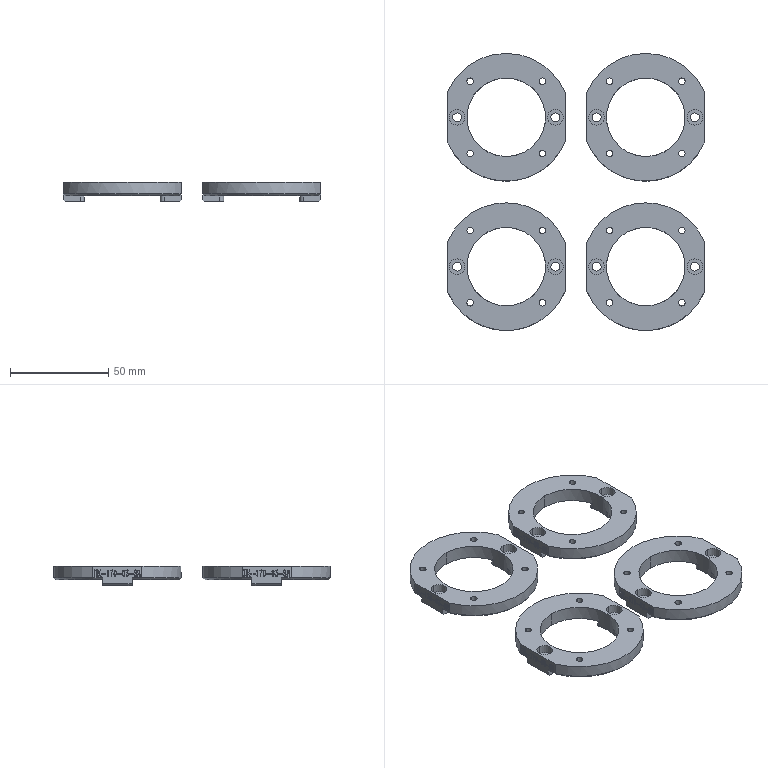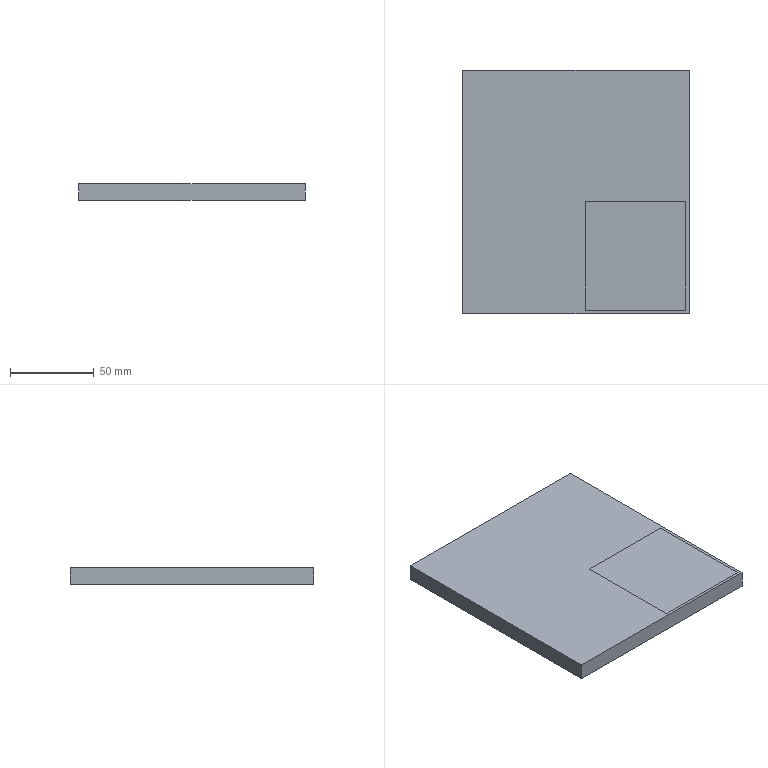CAM job | NX | 3-axis milling, drilling | part box 131 x 141 x 10 mm | stock box 135 x 145 x 10 mm
Tools:
number,name,description,diameter,corner_radius,flute_length,length,flutes
15,D10,Milling Tool-5 Parameters,10.0,0.0,50.0,75.0,2
14,D10JING,Milling Tool-5 Parameters,10.0,0.0,50.0,75.0,2
1,D6A45,Milling Tool-5 Parameters,6.0,0.0,50.0,75.0,2
8,4.5ZT,Drilling Tool,4.5,0.0,35.0,50.0,2
3,3.3ZT,Drilling Tool,3.3,0.0,35.0,50.0,2
12,D6,Milling Tool-5 Parameters,6.0,0.0,50.0,75.0,2
Operations:
program,operation,operation_type,tool,method,geometry_group,spindle_rpm,surface_speed,feed_per_tooth,feed_cut,feed_plunge,cut_length_mm,path_length_mm,cut_time_min,machine_time_min
1,ZLEVEL_PROFILE_COPY_1_COPY,ZLevelMilling,D10,METHOD,A,9500.0,298.0,0.1579,3000.0,1000.0,16139.625,16766.611,5.486,5.549
1,HOLE_MILLING,CylinderMilling,D10,METHOD,A,9500.0,298.0,0.1316,2500.0,1000.0,3694.87,4190.87,1.484,1.534
1,FLOOR_WALL,VolumeBased25DMillingOperation,D10,METHOD,A,9500.0,298.0,0.1579,3000.0,1000.0,8975.802,11210.784,3.043,3.266
1,FLOOR_WALL_COPY,VolumeBased25DMillingOperation,D10JING,METHOD,A,9500.0,298.0,0.0789,1500.0,1000.0,3437.242,6135.311,2.317,2.587
1,HOLE_MILLING_COPY,CylinderMilling,D10JING,METHOD,A,9500.0,298.0,0.0632,1200.0,1000.0,910.287,1406.287,0.7698,0.8194
1,DRILLING,Operation,D6A45,METHOD,A,5000.0,94.0,0.035,350.0,0.0,96.0,902.459,0.2743,0.3549
1,DRILLING_COPY,Operation,4.5ZT,METHOD,A,2000.0,40.0,0.075,300.0,0.0,114.816,629.476,0.3827,0.4342
1,DRILLING_COPY_COPY,Operation,3.3ZT,METHOD,A,2000.0,20.0,0.05,200.0,0.0,199.863,1056.434,0.9993,1.085
1,PLANAR_MILL_COPY_COPY_COPY_COPY,PlanarMilling,D6A45,METHOD,A,9500.0,179.0,0.0658,1250.0,100.0,584.616,1972.198,0.4677,0.6065
1,PLANAR_MILL_COPY_COPY_COPY_COPY_COPY,PlanarMilling,D6A45,METHOD,A,9500.0,179.0,0.0658,1250.0,100.0,160.755,966.023,0.1286,0.2091
1,PLANAR_MILL_COPY_COPY_COPY_COPY_COPY_COPY,PlanarMilling,D6A45,METHOD,A,9500.0,179.0,0.0658,1250.0,100.0,526.261,2799.275,0.421,0.6483
1,PLANAR_MILL_COPY_COPY_COPY_COPY_COPY_COPY_COPY,PlanarMilling,D6A45,METHOD,A,9500.0,179.0,0.0658,1250.0,100.0,699.471,1413.209,0.5596,0.631
1,ZLEVEL_PROFILE_COPY_1_COPY_COPY,ZLevelMilling,D10JING,METHOD,A,9500.0,298.0,0.0632,1200.0,1000.0,4715.232,5472.362,3.932,4.007
2,HOLE_MILLING_1,CylinderMilling,D6,METHOD,B,9500.0,179.0,0.0763,1450.0,100.0,142.389,320.189,0.0982,0.116
2,PLANAR_MILL_COPY_COPY_COPY_COPY_COPY_1,PlanarMilling,D6A45,METHOD,B,9500.0,179.0,0.0658,1250.0,100.0,401.972,1040.572,0.3216,0.3854